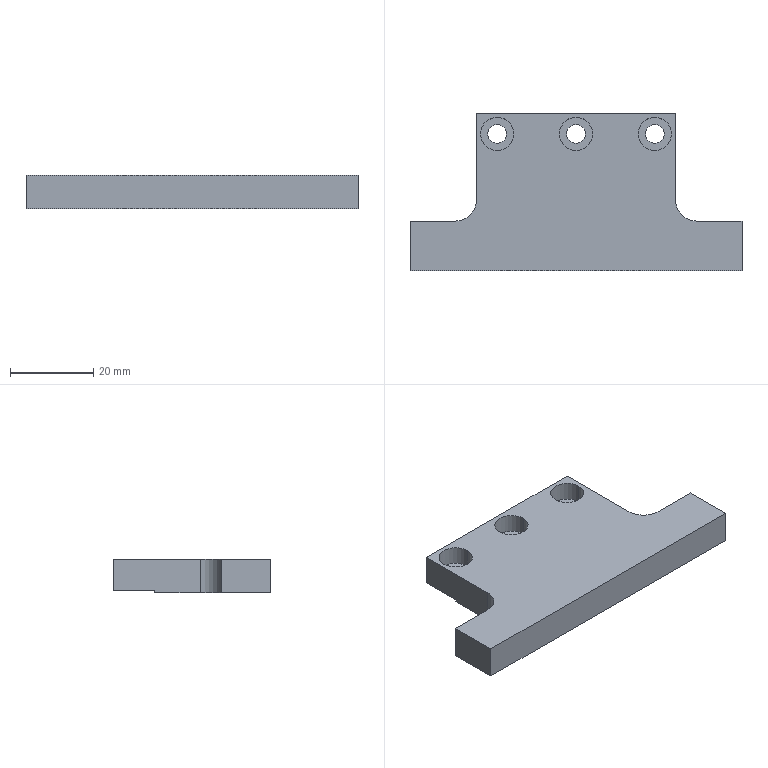Part | STEP file | 006 | 1 solid | 29 faces | box 80 x 38 x 8 mm | volume 16678 mm3 | plane 15 | cylinder 14 | commonest cylinder face diameters 4.5 x6 8 x6 10 x2